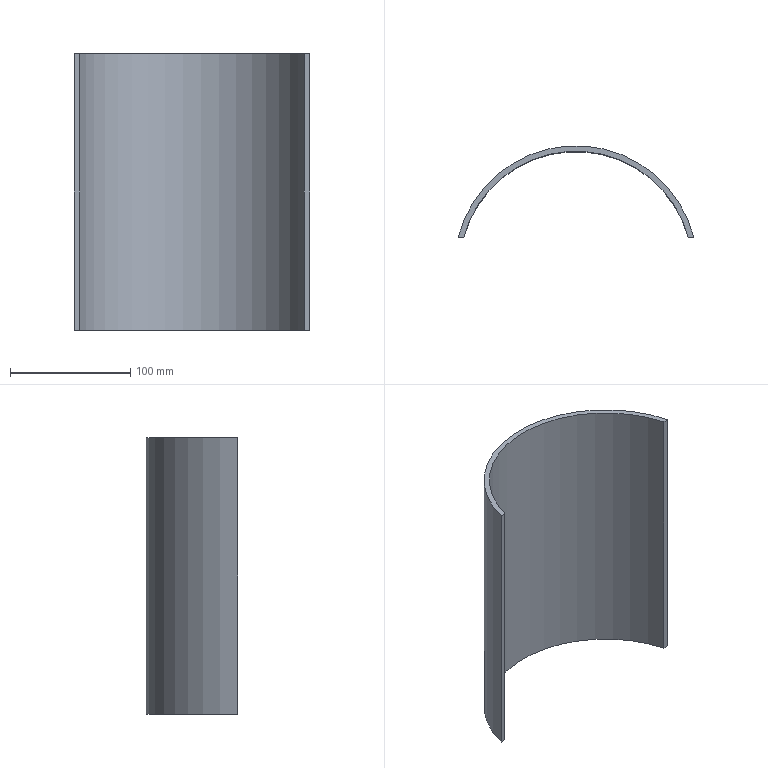Part | SolidWorks | features FlatPattern 1, ICE 1, SMBaseFlange 1, SheetMetal 1 | 1 solid | 6 faces | box 195.714 x 76 x 230 mm | volume 268771 mm3 | plane 4 | cylinder 2 | commonest cylinder face diameters 193 x1 202 x1
STEP:
#1=CARTESIAN_POINT('',(97.857,25.,230.));
#2=VERTEX_POINT('',#1);
#3=CARTESIAN_POINT('',(-97.857,25.,230.));
#4=VERTEX_POINT('',#3);
#5=CARTESIAN_POINT('',(0.,0.,230.));
#6=DIRECTION('',(0.,0.,1.));
#7=DIRECTION('',(1.,0.,0.));
#8=AXIS2_PLACEMENT_3D('',#5,#6,#7);
#9=CIRCLE('',#8,101.);
#10=EDGE_CURVE('',#2,#4,#9,.T.);
#11=ORIENTED_EDGE('',*,*,#10,.F.);
#12=CARTESIAN_POINT('',(97.857,25.,0.));
#13=VERTEX_POINT('',#12);
#14=CARTESIAN_POINT('',(97.857,25.,230.));
#15=DIRECTION('',(0.,0.,-1.));
#16=VECTOR('',#15,1000.);
#17=LINE('',#14,#16);
#18=EDGE_CURVE('',#2,#13,#17,.T.);
#19=ORIENTED_EDGE('',*,*,#18,.T.);
#20=CARTESIAN_POINT('',(-97.857,25.,0.));
#21=VERTEX_POINT('',#20);
#22=CARTESIAN_POINT('',(0.,0.,0.));
#23=DIRECTION('',(0.,0.,1.));
#24=DIRECTION('',(1.,0.,0.));
#25=AXIS2_PLACEMENT_3D('',#22,#23,#24);
#26=CIRCLE('',#25,101.);
#27=EDGE_CURVE('',#13,#21,#26,.T.);
#28=ORIENTED_EDGE('',*,*,#27,.T.);
#29=CARTESIAN_POINT('',(-97.857,25.,230.));
#30=DIRECTION('',(0.,0.,1.));
#31=VECTOR('',#30,1000.);
#32=LINE('',#29,#31);
#33=EDGE_CURVE('',#21,#4,#32,.T.);
#34=ORIENTED_EDGE('',*,*,#33,.T.);
#35=EDGE_LOOP('',(#11,#19,#28,#34));
#36=FACE_OUTER_BOUND('',#35,.T.);
#37=CARTESIAN_POINT('',(0.,0.,230.));
#38=DIRECTION('',(0.,0.,-1.));
#39=DIRECTION('',(-1.,0.,0.));
#40=AXIS2_PLACEMENT_3D('',#37,#38,#39);
#41=CYLINDRICAL_SURFACE('',#40,101.);
#42=ADVANCED_FACE('',(#36),#41,.T.);
#43=CARTESIAN_POINT('',(93.205,25.,230.));
#44=VERTEX_POINT('',#43);
#45=CARTESIAN_POINT('',(93.205,25.,0.));
#46=VERTEX_POINT('',#45);
#47=CARTESIAN_POINT('',(93.205,25.,230.));
#48=DIRECTION('',(0.,0.,-1.));
#49=VECTOR('',#48,1000.);
#50=LINE('',#47,#49);
#51=EDGE_CURVE('',#44,#46,#50,.T.);
#52=ORIENTED_EDGE('',*,*,#51,.F.);
#53=CARTESIAN_POINT('',(-93.205,25.,230.));
#54=VERTEX_POINT('',#53);
#55=CARTESIAN_POINT('',(0.,0.,230.));
#56=DIRECTION('',(0.,0.,1.));
#57=DIRECTION('',(1.,0.,0.));
#58=AXIS2_PLACEMENT_3D('',#55,#56,#57);
#59=CIRCLE('',#58,96.5);
#60=EDGE_CURVE('',#44,#54,#59,.T.);
#61=ORIENTED_EDGE('',*,*,#60,.T.);
#62=CARTESIAN_POINT('',(-93.205,25.,0.));
#63=VERTEX_POINT('',#62);
#64=CARTESIAN_POINT('',(-93.205,25.,230.));
#65=DIRECTION('',(0.,0.,1.));
#66=VECTOR('',#65,1000.);
#67=LINE('',#64,#66);
#68=EDGE_CURVE('',#63,#54,#67,.T.);
#69=ORIENTED_EDGE('',*,*,#68,.F.);
#70=CARTESIAN_POINT('',(0.,0.,0.));
#71=DIRECTION('',(0.,0.,1.));
#72=DIRECTION('',(1.,0.,0.));
#73=AXIS2_PLACEMENT_3D('',#70,#71,#72);
#74=CIRCLE('',#73,96.5);
#75=EDGE_CURVE('',#46,#63,#74,.T.);
#76=ORIENTED_EDGE('',*,*,#75,.F.);
#77=EDGE_LOOP('',(#52,#61,#69,#76));
#78=FACE_OUTER_BOUND('',#77,.T.);
#79=CARTESIAN_POINT('',(0.,0.,230.));
#80=DIRECTION('',(0.,0.,-1.));
#81=DIRECTION('',(-1.,0.,0.));
#82=AXIS2_PLACEMENT_3D('',#79,#80,#81);
#83=CYLINDRICAL_SURFACE('',#82,96.5);
#84=ADVANCED_FACE('',(#78),#83,.F.);
#85=CARTESIAN_POINT('',(-101.,25.,230.));
#86=DIRECTION('',(-1.,0.,0.));
#87=VECTOR('',#86,1000.);
#88=LINE('',#85,#87);
#89=EDGE_CURVE('',#2,#44,#88,.T.);
#90=ORIENTED_EDGE('',*,*,#89,.F.);
#91=ORIENTED_EDGE('',*,*,#10,.T.);
#92=CARTESIAN_POINT('',(-101.,25.,230.));
#93=DIRECTION('',(-1.,0.,0.));
#94=VECTOR('',#93,1000.);
#95=LINE('',#92,#94);
#96=EDGE_CURVE('',#54,#4,#95,.T.);
#97=ORIENTED_EDGE('',*,*,#96,.F.);
#98=ORIENTED_EDGE('',*,*,#60,.F.);
#99=EDGE_LOOP('',(#90,#91,#97,#98));
#100=FACE_OUTER_BOUND('',#99,.T.);
#101=CARTESIAN_POINT('',(0.,0.,230.));
#102=DIRECTION('',(0.,0.,1.));
#103=DIRECTION('',(1.,0.,0.));
#104=AXIS2_PLACEMENT_3D('',#101,#102,#103);
#105=PLANE('',#104);
#106=ADVANCED_FACE('',(#100),#105,.T.);
#107=ORIENTED_EDGE('',*,*,#27,.F.);
#108=CARTESIAN_POINT('',(0.,25.,0.));
#109=DIRECTION('',(-1.,0.,0.));
#110=VECTOR('',#109,1000.);
#111=LINE('',#108,#110);
#112=EDGE_CURVE('',#13,#46,#111,.T.);
#113=ORIENTED_EDGE('',*,*,#112,.T.);
#114=ORIENTED_EDGE('',*,*,#75,.T.);
#115=CARTESIAN_POINT('',(0.,25.,0.));
#116=DIRECTION('',(-1.,0.,0.));
#117=VECTOR('',#116,1000.);
#118=LINE('',#115,#117);
#119=EDGE_CURVE('',#63,#21,#118,.T.);
#120=ORIENTED_EDGE('',*,*,#119,.T.);
#121=EDGE_LOOP('',(#107,#113,#114,#120));
#122=FACE_OUTER_BOUND('',#121,.T.);
#123=CARTESIAN_POINT('',(0.,0.,0.));
#124=DIRECTION('',(0.,0.,1.));
#125=DIRECTION('',(1.,0.,0.));
#126=AXIS2_PLACEMENT_3D('',#123,#124,#125);
#127=PLANE('',#126);
#128=ADVANCED_FACE('',(#122),#127,.F.);
#129=ORIENTED_EDGE('',*,*,#119,.F.);
#130=ORIENTED_EDGE('',*,*,#68,.T.);
#131=ORIENTED_EDGE('',*,*,#96,.T.);
#132=ORIENTED_EDGE('',*,*,#33,.F.);
#133=EDGE_LOOP('',(#129,#130,#131,#132));
#134=FACE_OUTER_BOUND('',#133,.T.);
#135=CARTESIAN_POINT('',(-101.,25.,-72.));
#136=DIRECTION('',(0.,1.,0.));
#137=DIRECTION('',(0.,0.,1.));
#138=AXIS2_PLACEMENT_3D('',#135,#136,#137);
#139=PLANE('',#138);
#140=ADVANCED_FACE('',(#134),#139,.F.);
#141=ORIENTED_EDGE('',*,*,#89,.T.);
#142=ORIENTED_EDGE('',*,*,#51,.T.);
#143=ORIENTED_EDGE('',*,*,#112,.F.);
#144=ORIENTED_EDGE('',*,*,#18,.F.);
#145=EDGE_LOOP('',(#141,#142,#143,#144));
#146=FACE_OUTER_BOUND('',#145,.T.);
#147=CARTESIAN_POINT('',(-101.,25.,-72.));
#148=DIRECTION('',(0.,1.,0.));
#149=DIRECTION('',(0.,0.,1.));
#150=AXIS2_PLACEMENT_3D('',#147,#148,#149);
#151=PLANE('',#150);
#152=ADVANCED_FACE('',(#146),#151,.F.);
#153=CLOSED_SHELL('',(#42,#84,#106,#128,#140,#152));
#154=MANIFOLD_SOLID_BREP('',#153);
#155=CARTESIAN_POINT('',(0.,0.,0.));
#156=DIRECTION('',(0.,0.,1.));
#157=DIRECTION('',(1.,0.,0.));
#158=AXIS2_PLACEMENT_3D('',#155,#156,#157);
#159=(LENGTH_UNIT()NAMED_UNIT(*)SI_UNIT(.MILLI.,.METRE.));
#160=UNCERTAINTY_MEASURE_WITH_UNIT(LENGTH_MEASURE(0.00001),#159,'','');
#161=(NAMED_UNIT(*)PLANE_ANGLE_UNIT()SI_UNIT($,.RADIAN.));
#162=(NAMED_UNIT(*)SI_UNIT($,.STERADIAN.)SOLID_ANGLE_UNIT());
#163=(GEOMETRIC_REPRESENTATION_CONTEXT(3)GLOBAL_UNCERTAINTY_ASSIGNED_CONTEXT((#160))GLOBAL_UNIT_ASSIGNED_CONTEXT((#159,#161,#162))REPRESENTATION_CONTEXT('',''));
#164=ADVANCED_BREP_SHAPE_REPRESENTATION('',(#154,#158),#163);